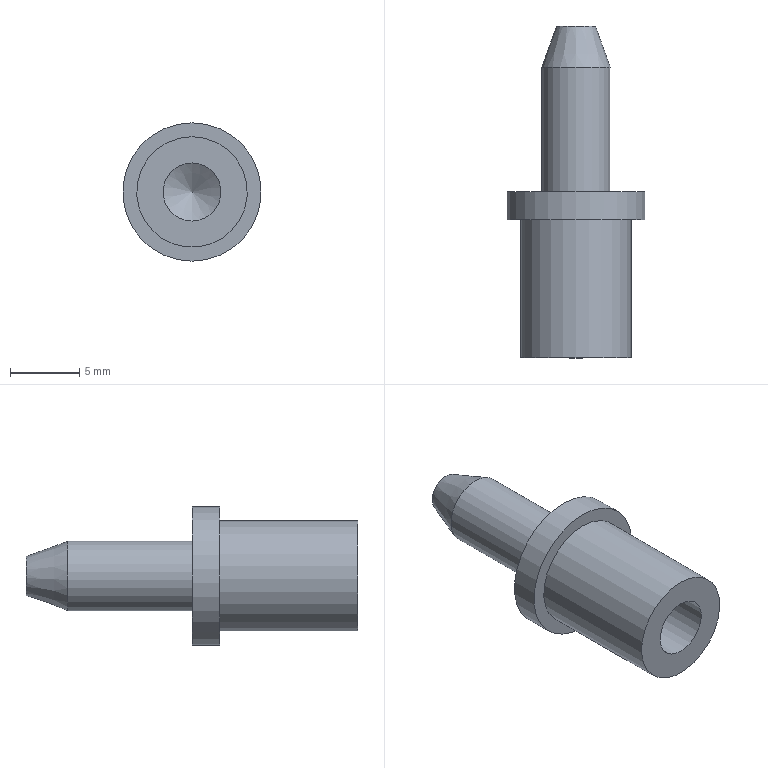Part | NX | features BREP 1 | 1 solid | 10 faces | box 10 x 24 x 10 mm | volume 695.75 mm3 | plane 4 | cylinder 4 | cone 2 | commonest cylinder face diameters 4.2 x1 5 x1 8 x1 10 x1
STEP:
#1=CARTESIAN_POINT('',(0.,0.,-2.1));
#2=VERTEX_POINT('',#1);
#3=CARTESIAN_POINT('',(0.,0.,0.));
#4=DIRECTION('',(0.,-1.,0.));
#5=DIRECTION('',(0.,0.,-1.));
#6=AXIS2_PLACEMENT_3D('',#3,#4,#5);
#7=CIRCLE('',#6,2.1);
#8=EDGE_CURVE('',#2,#2,#7,.T.);
#9=ORIENTED_EDGE('',*,*,#8,.F.);
#10=EDGE_LOOP('',(#9));
#11=FACE_BOUND('',#10,.T.);
#12=CARTESIAN_POINT('',(0.,0.,4.));
#13=VERTEX_POINT('',#12);
#14=CARTESIAN_POINT('',(0.,0.,0.));
#15=DIRECTION('',(0.,1.,0.));
#16=DIRECTION('',(0.,0.,1.));
#17=AXIS2_PLACEMENT_3D('',#14,#15,#16);
#18=CIRCLE('',#17,4.);
#19=EDGE_CURVE('',#13,#13,#18,.T.);
#20=ORIENTED_EDGE('',*,*,#19,.F.);
#21=EDGE_LOOP('',(#20));
#22=FACE_BOUND('',#21,.T.);
#23=CARTESIAN_POINT('',(0.,0.,0.));
#24=DIRECTION('',(0.,1.,0.));
#25=DIRECTION('',(0.,0.,-1.));
#26=AXIS2_PLACEMENT_3D('',#23,#24,#25);
#27=PLANE('',#26);
#28=ADVANCED_FACE('',(#11,#22),#27,.F.);
#29=CARTESIAN_POINT('',(0.,10.,4.));
#30=VERTEX_POINT('',#29);
#31=CARTESIAN_POINT('',(0.,10.,0.));
#32=DIRECTION('',(0.,1.,0.));
#33=DIRECTION('',(0.,0.,1.));
#34=AXIS2_PLACEMENT_3D('',#31,#32,#33);
#35=CIRCLE('',#34,4.);
#36=EDGE_CURVE('',#30,#30,#35,.T.);
#37=ORIENTED_EDGE('',*,*,#36,.F.);
#38=EDGE_LOOP('',(#37));
#39=FACE_BOUND('',#38,.T.);
#40=ORIENTED_EDGE('',*,*,#19,.T.);
#41=EDGE_LOOP('',(#40));
#42=FACE_BOUND('',#41,.T.);
#43=CARTESIAN_POINT('',(0.,0.,0.));
#44=DIRECTION('',(0.,1.,0.));
#45=DIRECTION('',(0.,0.,-1.));
#46=AXIS2_PLACEMENT_3D('',#43,#44,#45);
#47=CYLINDRICAL_SURFACE('',#46,4.);
#48=ADVANCED_FACE('',(#39,#42),#47,.T.);
#49=CARTESIAN_POINT('',(0.,10.,5.));
#50=VERTEX_POINT('',#49);
#51=CARTESIAN_POINT('',(0.,10.,0.));
#52=DIRECTION('',(0.,1.,0.));
#53=DIRECTION('',(0.,0.,1.));
#54=AXIS2_PLACEMENT_3D('',#51,#52,#53);
#55=CIRCLE('',#54,5.);
#56=EDGE_CURVE('',#50,#50,#55,.T.);
#57=ORIENTED_EDGE('',*,*,#56,.F.);
#58=EDGE_LOOP('',(#57));
#59=FACE_BOUND('',#58,.T.);
#60=ORIENTED_EDGE('',*,*,#36,.T.);
#61=EDGE_LOOP('',(#60));
#62=FACE_BOUND('',#61,.T.);
#63=CARTESIAN_POINT('',(4.,10.,0.));
#64=DIRECTION('',(0.,1.,0.));
#65=DIRECTION('',(0.,0.,-1.));
#66=AXIS2_PLACEMENT_3D('',#63,#64,#65);
#67=PLANE('',#66);
#68=ADVANCED_FACE('',(#59,#62),#67,.F.);
#69=CARTESIAN_POINT('',(0.,12.,5.));
#70=VERTEX_POINT('',#69);
#71=CARTESIAN_POINT('',(0.,12.,0.));
#72=DIRECTION('',(0.,1.,0.));
#73=DIRECTION('',(0.,0.,1.));
#74=AXIS2_PLACEMENT_3D('',#71,#72,#73);
#75=CIRCLE('',#74,5.);
#76=EDGE_CURVE('',#70,#70,#75,.T.);
#77=ORIENTED_EDGE('',*,*,#76,.F.);
#78=EDGE_LOOP('',(#77));
#79=FACE_BOUND('',#78,.T.);
#80=ORIENTED_EDGE('',*,*,#56,.T.);
#81=EDGE_LOOP('',(#80));
#82=FACE_BOUND('',#81,.T.);
#83=CARTESIAN_POINT('',(0.,0.,0.));
#84=DIRECTION('',(0.,1.,0.));
#85=DIRECTION('',(0.,0.,-1.));
#86=AXIS2_PLACEMENT_3D('',#83,#84,#85);
#87=CYLINDRICAL_SURFACE('',#86,5.);
#88=ADVANCED_FACE('',(#79,#82),#87,.T.);
#89=CARTESIAN_POINT('',(0.,12.,2.5));
#90=VERTEX_POINT('',#89);
#91=CARTESIAN_POINT('',(0.,12.,0.));
#92=DIRECTION('',(0.,1.,0.));
#93=DIRECTION('',(0.,0.,1.));
#94=AXIS2_PLACEMENT_3D('',#91,#92,#93);
#95=CIRCLE('',#94,2.5);
#96=EDGE_CURVE('',#90,#90,#95,.T.);
#97=ORIENTED_EDGE('',*,*,#96,.F.);
#98=EDGE_LOOP('',(#97));
#99=FACE_BOUND('',#98,.T.);
#100=ORIENTED_EDGE('',*,*,#76,.T.);
#101=EDGE_LOOP('',(#100));
#102=FACE_BOUND('',#101,.T.);
#103=CARTESIAN_POINT('',(5.,12.,0.));
#104=DIRECTION('',(0.,-1.,0.));
#105=DIRECTION('',(0.,0.,1.));
#106=AXIS2_PLACEMENT_3D('',#103,#104,#105);
#107=PLANE('',#106);
#108=ADVANCED_FACE('',(#99,#102),#107,.F.);
#109=CARTESIAN_POINT('',(0.,21.,2.5));
#110=VERTEX_POINT('',#109);
#111=CARTESIAN_POINT('',(0.,21.,0.));
#112=DIRECTION('',(0.,1.,0.));
#113=DIRECTION('',(0.,0.,1.));
#114=AXIS2_PLACEMENT_3D('',#111,#112,#113);
#115=CIRCLE('',#114,2.5);
#116=EDGE_CURVE('',#110,#110,#115,.T.);
#117=ORIENTED_EDGE('',*,*,#116,.F.);
#118=EDGE_LOOP('',(#117));
#119=FACE_BOUND('',#118,.T.);
#120=ORIENTED_EDGE('',*,*,#96,.T.);
#121=EDGE_LOOP('',(#120));
#122=FACE_BOUND('',#121,.T.);
#123=CARTESIAN_POINT('',(0.,0.,0.));
#124=DIRECTION('',(0.,1.,0.));
#125=DIRECTION('',(0.,0.,-1.));
#126=AXIS2_PLACEMENT_3D('',#123,#124,#125);
#127=CYLINDRICAL_SURFACE('',#126,2.5);
#128=ADVANCED_FACE('',(#119,#122),#127,.T.);
#129=CARTESIAN_POINT('',(0.,24.,1.408));
#130=VERTEX_POINT('',#129);
#131=CARTESIAN_POINT('',(0.,24.,0.));
#132=DIRECTION('',(0.,1.,0.));
#133=DIRECTION('',(0.,0.,1.));
#134=AXIS2_PLACEMENT_3D('',#131,#132,#133);
#135=CIRCLE('',#134,1.408);
#136=EDGE_CURVE('',#130,#130,#135,.T.);
#137=ORIENTED_EDGE('',*,*,#136,.F.);
#138=EDGE_LOOP('',(#137));
#139=FACE_BOUND('',#138,.T.);
#140=ORIENTED_EDGE('',*,*,#116,.T.);
#141=EDGE_LOOP('',(#140));
#142=FACE_BOUND('',#141,.T.);
#143=CARTESIAN_POINT('',(0.,21.,0.));
#144=DIRECTION('',(0.,-1.,0.));
#145=DIRECTION('',(0.,0.,1.));
#146=AXIS2_PLACEMENT_3D('',#143,#144,#145);
#147=CONICAL_SURFACE('',#146,2.5,0.3491);
#148=ADVANCED_FACE('',(#139,#142),#147,.T.);
#149=ORIENTED_EDGE('',*,*,#136,.T.);
#150=EDGE_LOOP('',(#149));
#151=FACE_BOUND('',#150,.T.);
#152=CARTESIAN_POINT('',(1.408,24.,0.));
#153=DIRECTION('',(0.,-1.,0.));
#154=DIRECTION('',(0.,0.,1.));
#155=AXIS2_PLACEMENT_3D('',#152,#153,#154);
#156=PLANE('',#155);
#157=ADVANCED_FACE('',(#151),#156,.F.);
#158=CARTESIAN_POINT('',(0.,13.662,0.));
#159=VERTEX_POINT('',#158);
#160=VERTEX_LOOP('',#159);
#161=FACE_BOUND('',#160,.T.);
#162=CARTESIAN_POINT('',(0.,12.4,-2.1));
#163=VERTEX_POINT('',#162);
#164=CARTESIAN_POINT('',(0.,12.4,0.));
#165=DIRECTION('',(0.,-1.,0.));
#166=DIRECTION('',(0.,0.,-1.));
#167=AXIS2_PLACEMENT_3D('',#164,#165,#166);
#168=CIRCLE('',#167,2.1);
#169=EDGE_CURVE('',#163,#163,#168,.T.);
#170=ORIENTED_EDGE('',*,*,#169,.T.);
#171=EDGE_LOOP('',(#170));
#172=FACE_BOUND('',#171,.T.);
#173=CARTESIAN_POINT('',(0.,12.4,0.));
#174=DIRECTION('',(0.,-1.,0.));
#175=DIRECTION('',(0.,0.,1.));
#176=AXIS2_PLACEMENT_3D('',#173,#174,#175);
#177=CONICAL_SURFACE('',#176,2.1,1.03);
#178=ADVANCED_FACE('',(#161,#172),#177,.F.);
#179=ORIENTED_EDGE('',*,*,#169,.F.);
#180=EDGE_LOOP('',(#179));
#181=FACE_BOUND('',#180,.T.);
#182=ORIENTED_EDGE('',*,*,#8,.T.);
#183=EDGE_LOOP('',(#182));
#184=FACE_BOUND('',#183,.T.);
#185=CARTESIAN_POINT('',(0.,0.,0.));
#186=DIRECTION('',(0.,-1.,0.));
#187=DIRECTION('',(0.,0.,1.));
#188=AXIS2_PLACEMENT_3D('',#185,#186,#187);
#189=CYLINDRICAL_SURFACE('',#188,2.1);
#190=ADVANCED_FACE('',(#181,#184),#189,.F.);
#191=CLOSED_SHELL('',(#28,#48,#68,#88,#108,#128,#148,#157,#178,#190));
#192=MANIFOLD_SOLID_BREP('',#191);
#193=(LENGTH_UNIT()NAMED_UNIT(*)SI_UNIT(.MILLI.,.METRE.));
#194=UNCERTAINTY_MEASURE_WITH_UNIT(LENGTH_MEASURE(0.00001),#193,'','');
#195=(NAMED_UNIT(*)PLANE_ANGLE_UNIT()SI_UNIT($,.RADIAN.));
#196=(NAMED_UNIT(*)SI_UNIT($,.STERADIAN.)SOLID_ANGLE_UNIT());
#197=(GEOMETRIC_REPRESENTATION_CONTEXT(3)GLOBAL_UNCERTAINTY_ASSIGNED_CONTEXT((#194))GLOBAL_UNIT_ASSIGNED_CONTEXT((#193,#195,#196))REPRESENTATION_CONTEXT('',''));
#198=ADVANCED_BREP_SHAPE_REPRESENTATION('',(#192),#197);